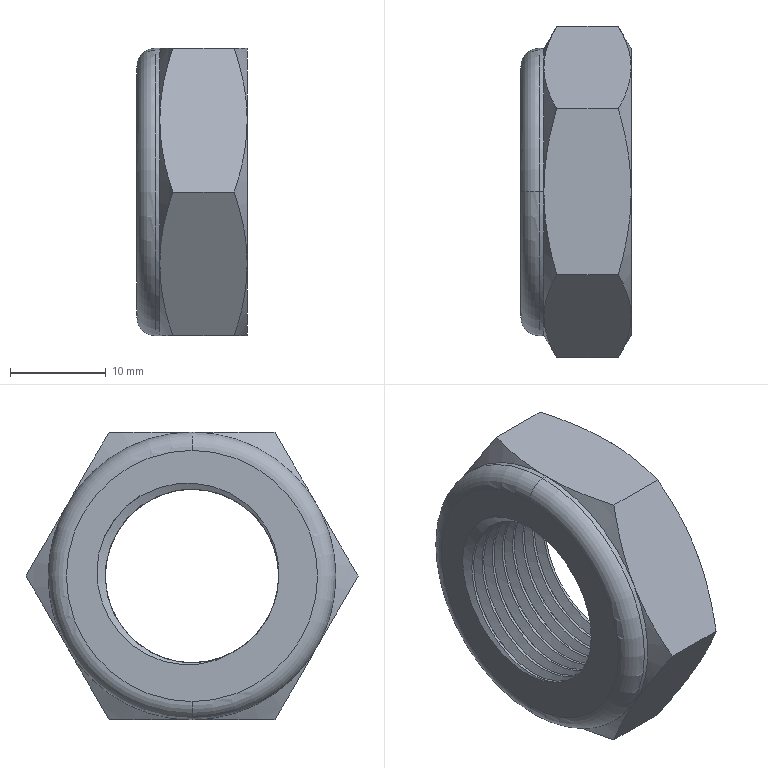Part | STEP file | Completa.sldasm-Part-116_Valor predeterminado | 1 solid | 60 faces | box 11.5 x 34.641 x 30 mm | volume 5406 mm3 | cylinder 36 | cone 12 | plane 8 | torus 2 | spline 2 | commonest cylinder face diameters 18.1 x17 20 x17 30 x2